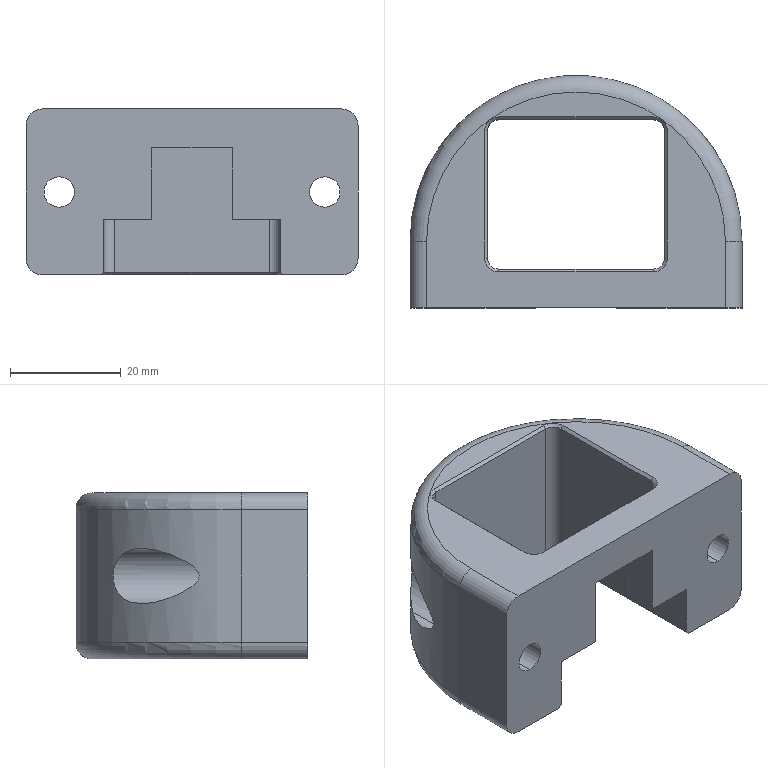Part | SolidWorks | features Fillet 2, ICE 2, Chamfer 1, Extrusion 1, HoleWzd 1 | 1 solid | 48 faces | box 60 x 42 x 30 mm | volume 30390 mm3 | plane 23 | cylinder 17 | cone 6 | torus 2 | commonest cylinder face diameters 4 x4 5.5 x4 6 x4 10 x4 60 x1